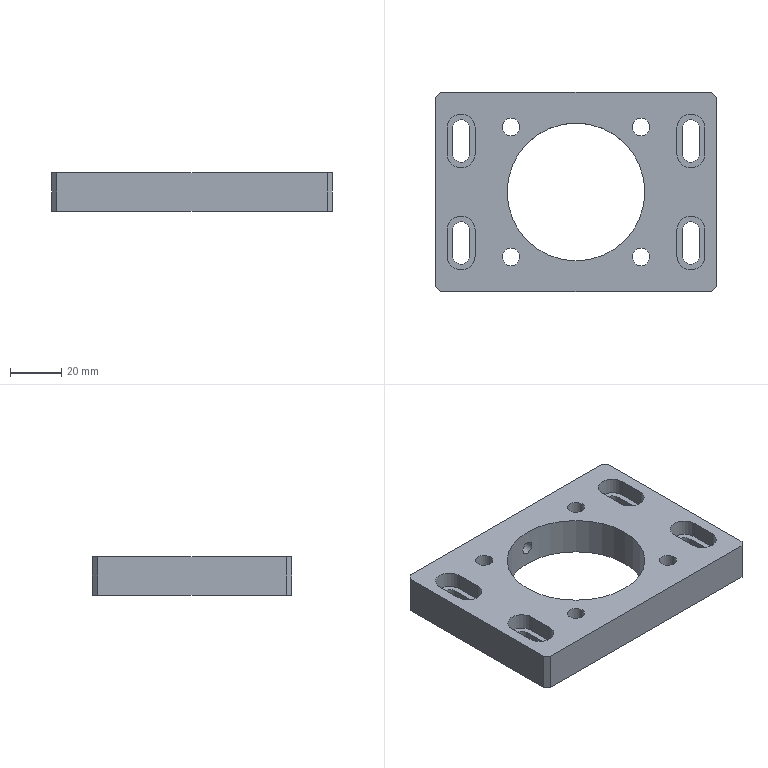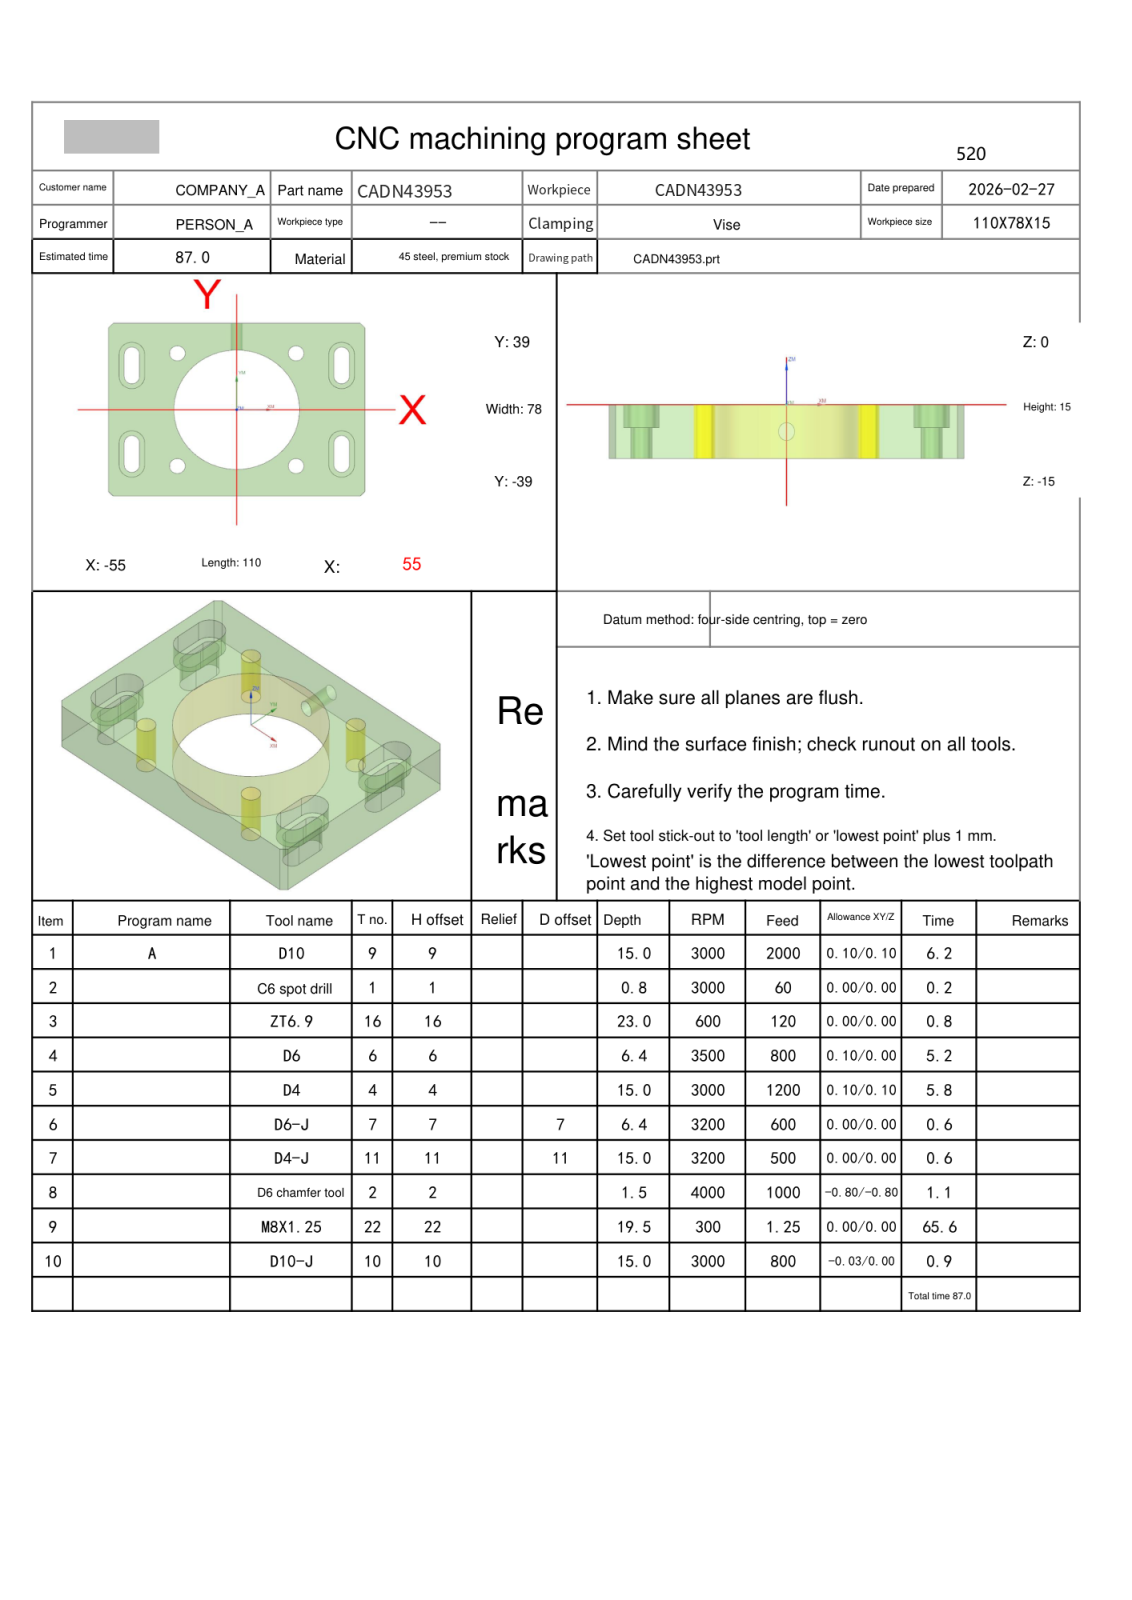NC program | NX | posted by the shop | part box 110 x 78 x 15 mm
Lines 1 to 1524 of 4469:
%
O0001
(Machine time: 151.17 MIN)
(===Total Tool:10===)
(T9=D10     D=10.  R=0.   D-  H09 Z=-15.  )
(T1=C6 spot drill   D=6.   R=0.   D-  H01 Z=-0.8  )
(T16=ZT6.9  D=6.9  DR_a=120 D-  H16 Z=-23.  )
(T6=D6      D=6.   R=0.   D-  H06 Z=-6.4  )
(T4=D4      D=4.   R=0.   D-  H04 Z=-15.  )
(T7=D6-J    D=6.   R=0.   D7  H07 Z=-6.4  )
(T11=D4-J   D=4.   R=0.   D11 H11 Z=-15.  )
(T2=D6 chamfer tool   D=6.   R=0.   D-  H02 Z=-1.5  )
(T22=M8X1.25 D=6.8  DR_a=180 D-  H22 Z=-19.5 )
(T10=D10-J  D=10.  R=0.   D10 H10 Z=-15.  )
G80 G90 G17 G49 G40
G91 G28 Z0
M01
N1 T09 M06
(D10  D=10. R=0. H=09 ce=0.10 di=0.10)
G00 G90 G54 X-50.242 Y-48.97 M03 S3000
G43 H09 Z50.
M08
Z-.5
G01 X-56.606 Y-42.606 F2000.
X-58.606 Y-40.606
X-64.97 Y-34.242
G00 Z-1.
G01 X-58.606 Y-40.606
X-56.606 Y-42.606
X-50.242 Y-48.97
G00 Z-1.5
G01 X-56.606 Y-42.606
X-58.606 Y-40.606
X-64.97 Y-34.242
G00 Z-2.
G01 X-58.606 Y-40.606
X-56.606 Y-42.606
X-50.242 Y-48.97
G00 Z-2.5
G01 X-56.606 Y-42.606
X-58.606 Y-40.606
X-64.97 Y-34.242
G00 Z-3.
G01 X-58.606 Y-40.606
X-56.606 Y-42.606
X-50.242 Y-48.97
G00 Z-3.5
G01 X-56.606 Y-42.606
X-58.606 Y-40.606
X-64.97 Y-34.242
G00 Z-4.
G01 X-58.606 Y-40.606
X-56.606 Y-42.606
X-50.242 Y-48.97
G00 Z-4.5
G01 X-56.606 Y-42.606
X-58.606 Y-40.606
X-64.97 Y-34.242
G00 Z-5.
G01 X-58.606 Y-40.606
X-56.606 Y-42.606
X-50.242 Y-48.97
G00 Z-5.5
G01 X-56.606 Y-42.606
X-58.606 Y-40.606
X-64.97 Y-34.242
G00 Z-6.
G01 X-58.606 Y-40.606
X-56.606 Y-42.606
X-50.242 Y-48.97
G00 Z-6.5
G01 X-56.606 Y-42.606
X-58.606 Y-40.606
X-64.97 Y-34.242
G00 Z-7.
G01 X-58.606 Y-40.606
X-56.606 Y-42.606
X-50.242 Y-48.97
G00 Z-7.5
G01 X-56.606 Y-42.606
X-58.606 Y-40.606
X-64.97 Y-34.242
G00 Z-7.9
G01 X-58.606 Y-40.606
X-56.606 Y-42.606
X-50.242 Y-48.97
G00 Z50.
X-64.97 Y34.242
Z-.5
G01 X-58.606 Y40.606
X-56.606 Y42.606
X-50.242 Y48.97
G00 Z-1.
G01 X-56.606 Y42.606
X-58.606 Y40.606
X-64.97 Y34.242
G00 Z-1.5
G01 X-58.606 Y40.606
X-56.606 Y42.606
X-50.242 Y48.97
G00 Z-2.
G01 X-56.606 Y42.606
X-58.606 Y40.606
X-64.97 Y34.242
G00 Z-2.5
G01 X-58.606 Y40.606
X-56.606 Y42.606
X-50.242 Y48.97
G00 Z-3.
G01 X-56.606 Y42.606
X-58.606 Y40.606
X-64.97 Y34.242
G00 Z-3.5
G01 X-58.606 Y40.606
X-56.606 Y42.606
X-50.242 Y48.97
G00 Z-4.
G01 X-56.606 Y42.606
X-58.606 Y40.606
X-64.97 Y34.242
G00 Z-4.5
G01 X-58.606 Y40.606
X-56.606 Y42.606
X-50.242 Y48.97
G00 Z-5.
G01 X-56.606 Y42.606
X-58.606 Y40.606
X-64.97 Y34.242
G00 Z-5.5
G01 X-58.606 Y40.606
X-56.606 Y42.606
X-50.242 Y48.97
G00 Z-6.
G01 X-56.606 Y42.606
X-58.606 Y40.606
X-64.97 Y34.242
G00 Z-6.5
G01 X-58.606 Y40.606
X-56.606 Y42.606
X-50.242 Y48.97
G00 Z-7.
G01 X-56.606 Y42.606
X-58.606 Y40.606
X-64.97 Y34.242
G00 Z-7.5
G01 X-58.606 Y40.606
X-56.606 Y42.606
X-50.242 Y48.97
G00 Z-7.9
G01 X-56.606 Y42.606
X-58.606 Y40.606
X-64.97 Y34.242
G00 Z50.
X50.242 Y48.97
Z-.5
G01 X56.606 Y42.606
X58.606 Y40.606
X64.97 Y34.242
G00 Z-1.
G01 X58.606 Y40.606
X56.606 Y42.606
X50.242 Y48.97
G00 Z-1.5
G01 X56.606 Y42.606
X58.606 Y40.606
X64.97 Y34.242
G00 Z-2.
G01 X58.606 Y40.606
X56.606 Y42.606
X50.242 Y48.97
G00 Z-2.5
G01 X56.606 Y42.606
X58.606 Y40.606
X64.97 Y34.242
G00 Z-3.
G01 X58.606 Y40.606
X56.606 Y42.606
X50.242 Y48.97
G00 Z-3.5
G01 X56.606 Y42.606
X58.606 Y40.606
X64.97 Y34.242
G00 Z-4.
G01 X58.606 Y40.606
X56.606 Y42.606
X50.242 Y48.97
G00 Z-4.5
G01 X56.606 Y42.606
X58.606 Y40.606
X64.97 Y34.242
G00 Z-5.
G01 X58.606 Y40.606
X56.606 Y42.606
X50.242 Y48.97
G00 Z-5.5
G01 X56.606 Y42.606
X58.606 Y40.606
X64.97 Y34.242
G00 Z-6.
G01 X58.606 Y40.606
X56.606 Y42.606
X50.242 Y48.97
G00 Z-6.5
G01 X56.606 Y42.606
X58.606 Y40.606
X64.97 Y34.242
G00 Z-7.
G01 X58.606 Y40.606
X56.606 Y42.606
X50.242 Y48.97
G00 Z-7.5
G01 X56.606 Y42.606
X58.606 Y40.606
X64.97 Y34.242
G00 Z-7.9
G01 X58.606 Y40.606
X56.606 Y42.606
X50.242 Y48.97
G00 Z50.
X64.97 Y-34.242
Z-.5
G01 X58.606 Y-40.606
X56.606 Y-42.606
X50.242 Y-48.97
G00 Z-1.
G01 X56.606 Y-42.606
X58.606 Y-40.606
X64.97 Y-34.242
G00 Z-1.5
G01 X58.606 Y-40.606
X56.606 Y-42.606
X50.242 Y-48.97
G00 Z-2.
G01 X56.606 Y-42.606
X58.606 Y-40.606
X64.97 Y-34.242
G00 Z-2.5
G01 X58.606 Y-40.606
X56.606 Y-42.606
X50.242 Y-48.97
G00 Z-3.
G01 X56.606 Y-42.606
X58.606 Y-40.606
X64.97 Y-34.242
G00 Z-3.5
G01 X58.606 Y-40.606
X56.606 Y-42.606
X50.242 Y-48.97
G00 Z-4.
G01 X56.606 Y-42.606
X58.606 Y-40.606
X64.97 Y-34.242
G00 Z-4.5
G01 X58.606 Y-40.606
X56.606 Y-42.606
X50.242 Y-48.97
G00 Z-5.
G01 X56.606 Y-42.606
X58.606 Y-40.606
X64.97 Y-34.242
G00 Z-5.5
G01 X58.606 Y-40.606
X56.606 Y-42.606
X50.242 Y-48.97
G00 Z-6.
G01 X56.606 Y-42.606
X58.606 Y-40.606
X64.97 Y-34.242
G00 Z-6.5
G01 X58.606 Y-40.606
X56.606 Y-42.606
X50.242 Y-48.97
G00 Z-7.
G01 X56.606 Y-42.606
X58.606 Y-40.606
X64.97 Y-34.242
G00 Z-7.5
G01 X58.606 Y-40.606
X56.606 Y-42.606
X50.242 Y-48.97
G00 Z-7.9
G01 X56.606 Y-42.606
X58.606 Y-40.606
X64.97 Y-34.242
G00 Z50.
G00 G90 X-1.466 Y12.145 M03 S3000
Z10.1
Z1.5
G02 X-1.466 Y12.145 Z.018 I1.466 J4.255 F2000.
X-2.587 Y20.082 Z-.5 I1.466 J4.255
G01 X0.0 Y21.9
G02 X21.9 Y0.0 I0.0 J-21.9
X0.0 Y-21.9 I-21.9 J0.0
X-21.9 Y0.0 I0.0 J21.9
X0.0 Y21.9 I21.9 J0.0
X4.957 Y21.332 I0.0 J-21.9
X5.73 Y20.36 I-.226 J-.974
G01 X5.747 Y14.394
G03 X6.322 Y13.492 I1. J.003
G02 X14.9 Y0.0 I-6.322 J-13.492
X0.0 Y-14.9 I-14.9 J0.0
X-14.9 Y0.0 I0.0 J14.9
X0.0 Y14.9 I14.9 J0.0
X.225 Y14.898 I0.0 J-14.9
X1.14 Y14.265 I-.015 J-1.
G01 X3.975 Y7.06
G03 X4.354 Y6.592 I.93 J.366
G02 X7.9 Y0.0 I-4.354 J-6.592
X0.0 Y-7.9 I-7.9 J0.0
X-7.9 Y0.0 I0.0 J7.9
X-1.587 Y7.739 I7.9 J0.0
G01 X-1.407 Y7.757
G02 X-.525 Y7.038 I0.0 J-.9
G01 X.873 Y.224
X.88 Y.19
X.9 Y0.0
G02 X0.0 Y-.9 I-.9 J0.0
X-.9 Y0.0 I0.0 J.9
X0.0 Y.9 I.9 J0.0
X.204 Y.877 I0.0 J-.9
X.635 Y.637 I-.204 J-.877
G03 X5.578 Y-1.405 I4.942 J4.957
X10.535 Y.653 I0.0 J7.
G01 Z.7
G00 Z3.
G01 X-1.466 Y12.145 F6000.
G00 Z1.
G02 X-1.466 Y12.145 Z-.482 I1.466 J4.255 F2000.
X-2.587 Y20.082 Z-1. I1.466 J4.255
G01 X0.0 Y21.9
G02 X21.9 Y0.0 I0.0 J-21.9
X0.0 Y-21.9 I-21.9 J0.0
X-21.9 Y0.0 I0.0 J21.9
X0.0 Y21.9 I21.9 J0.0
X4.957 Y21.332 I0.0 J-21.9
X5.73 Y20.36 I-.226 J-.974
G01 X5.747 Y14.394
G03 X6.322 Y13.492 I1. J.003
G02 X14.9 Y0.0 I-6.322 J-13.492
X0.0 Y-14.9 I-14.9 J0.0
X-14.9 Y0.0 I0.0 J14.9
X0.0 Y14.9 I14.9 J0.0
X.225 Y14.898 I0.0 J-14.9
X1.14 Y14.265 I-.015 J-1.
G01 X3.975 Y7.06
G03 X4.354 Y6.592 I.93 J.366
G02 X7.9 Y0.0 I-4.354 J-6.592
X0.0 Y-7.9 I-7.9 J0.0
X-7.9 Y0.0 I0.0 J7.9
X-1.587 Y7.739 I7.9 J0.0
G01 X-1.407 Y7.757
G02 X-.525 Y7.038 I0.0 J-.9
G01 X.873 Y.224
X.88 Y.19
X.9 Y0.0
G02 X0.0 Y-.9 I-.9 J0.0
X-.9 Y0.0 I0.0 J.9
X0.0 Y.9 I.9 J0.0
X.204 Y.877 I0.0 J-.9
X.635 Y.637 I-.204 J-.877
G03 X5.578 Y-1.405 I4.942 J4.957
X10.535 Y.653 I0.0 J7.
G01 Z.2
G00 Z2.5
G01 X-1.466 Y12.145 F6000.
G00 Z.5
G02 X-1.466 Y12.145 Z-.982 I1.466 J4.255 F2000.
X-2.587 Y20.082 Z-1.5 I1.466 J4.255
G01 X0.0 Y21.9
G02 X21.9 Y0.0 I0.0 J-21.9
X0.0 Y-21.9 I-21.9 J0.0
X-21.9 Y0.0 I0.0 J21.9
X0.0 Y21.9 I21.9 J0.0
X4.957 Y21.332 I0.0 J-21.9
X5.73 Y20.36 I-.226 J-.974
G01 X5.747 Y14.394
G03 X6.322 Y13.492 I1. J.003
G02 X14.9 Y0.0 I-6.322 J-13.492
X0.0 Y-14.9 I-14.9 J0.0
X-14.9 Y0.0 I0.0 J14.9
X0.0 Y14.9 I14.9 J0.0
X.225 Y14.898 I0.0 J-14.9
X1.14 Y14.265 I-.015 J-1.
G01 X3.975 Y7.06
G03 X4.354 Y6.592 I.93 J.366
G02 X7.9 Y0.0 I-4.354 J-6.592
X0.0 Y-7.9 I-7.9 J0.0
X-7.9 Y0.0 I0.0 J7.9
X-1.587 Y7.739 I7.9 J0.0
G01 X-1.407 Y7.757
G02 X-.525 Y7.038 I0.0 J-.9
G01 X.872 Y.225
X.88 Y.19
X.9 Y0.0
G02 X0.0 Y-.9 I-.9 J0.0
X-.9 Y0.0 I0.0 J.9
X0.0 Y.9 I.9 J0.0
X.204 Y.877 I0.0 J-.9
G01 X.265 Y.86
G02 X.635 Y.637 I-.265 J-.86
G03 X5.578 Y-1.405 I4.942 J4.957
X10.535 Y.653 I0.0 J7.
G01 Z-.3
G00 Z2.
G01 X-1.466 Y12.145 F6000.
G00 Z0.0
G02 X-1.466 Y12.145 Z-1.482 I1.466 J4.255 F2000.
X-2.587 Y20.082 Z-2. I1.466 J4.255
G01 X0.0 Y21.9
G02 X21.9 Y0.0 I0.0 J-21.9
X0.0 Y-21.9 I-21.9 J0.0
X-21.9 Y0.0 I0.0 J21.9
X0.0 Y21.9 I21.9 J0.0
X4.957 Y21.332 I0.0 J-21.9
X5.73 Y20.36 I-.226 J-.974
G01 X5.747 Y14.394
G03 X6.322 Y13.492 I1. J.003
G02 X14.9 Y0.0 I-6.322 J-13.492
X0.0 Y-14.9 I-14.9 J0.0
X-14.9 Y0.0 I0.0 J14.9
X0.0 Y14.9 I14.9 J0.0
X.225 Y14.898 I0.0 J-14.9
X1.14 Y14.265 I-.015 J-1.
G01 X3.975 Y7.06
G03 X4.354 Y6.592 I.93 J.366
G02 X7.9 Y0.0 I-4.354 J-6.592
X0.0 Y-7.9 I-7.9 J0.0
X-7.9 Y0.0 I0.0 J7.9
X-1.651 Y7.725 I7.9 J0.0
G01 X-1.464 Y7.745
G02 X-.572 Y6.968 I0.0 J-.9
G01 X.095 Y2.097
G03 X.727 Y.531 I3.422 J.469
G02 X.9 Y0.0 I-.727 J-.531
X0.0 Y-.9 I-.9 J0.0
X-.9 Y0.0 I0.0 J.9
X0.0 Y.9 I.9 J0.0
X.204 Y.877 I0.0 J-.9
G01 X.265 Y.86
G02 X.635 Y.637 I-.265 J-.86
G03 X5.578 Y-1.405 I4.942 J4.957
X10.535 Y.653 I0.0 J7.
G01 Z-.8
G00 Z1.5
G01 X-1.466 Y12.145 F6000.
G00 Z-.5
G02 X-1.466 Y12.145 Z-1.982 I1.466 J4.255 F2000.
X-2.587 Y20.082 Z-2.5 I1.466 J4.255
G01 X0.0 Y21.9
G02 X21.9 Y0.0 I0.0 J-21.9
X0.0 Y-21.9 I-21.9 J0.0
X-21.9 Y0.0 I0.0 J21.9
X0.0 Y21.9 I21.9 J0.0
X4.957 Y21.332 I0.0 J-21.9
X5.73 Y20.36 I-.226 J-.974
G01 X5.747 Y14.394
G03 X6.322 Y13.492 I1. J.003
G02 X14.9 Y0.0 I-6.322 J-13.492
X0.0 Y-14.9 I-14.9 J0.0
X-14.9 Y0.0 I0.0 J14.9
X0.0 Y14.9 I14.9 J0.0
X.225 Y14.898 I0.0 J-14.9
X1.14 Y14.265 I-.015 J-1.
G01 X3.975 Y7.06
G03 X4.354 Y6.592 I.93 J.366
G02 X7.9 Y0.0 I-4.354 J-6.592
X0.0 Y-7.9 I-7.9 J0.0
X-7.9 Y0.0 I0.0 J7.9
X-1.628 Y7.731 I7.9 J0.0
G01 X-1.442 Y7.75
G02 X-.554 Y6.994 I0.0 J-.9
G01 X.295 Y1.737
G03 X.766 Y.473 I3.41 J.551
G02 X.9 Y0.0 I-.766 J-.473
X0.0 Y-.9 I-.9 J0.0
X-.9 Y0.0 I0.0 J.9
X0.0 Y.9 I.9 J0.0
X.204 Y.877 I0.0 J-.9
G01 X.265 Y.86
G02 X.635 Y.637 I-.265 J-.86
G03 X5.578 Y-1.405 I4.942 J4.957
X10.535 Y.653 I0.0 J7.
G01 Z-1.3
G00 Z1.
G01 X-1.466 Y12.145 F6000.
G00 Z-1.
G02 X-1.466 Y12.145 Z-2.482 I1.466 J4.255 F2000.
X-2.587 Y20.082 Z-3. I1.466 J4.255
G01 X0.0 Y21.9
G02 X21.9 Y0.0 I0.0 J-21.9
X0.0 Y-21.9 I-21.9 J0.0
X-21.9 Y0.0 I0.0 J21.9
X0.0 Y21.9 I21.9 J0.0
X4.957 Y21.332 I0.0 J-21.9
X5.73 Y20.36 I-.226 J-.974
G01 X5.747 Y14.394
G03 X6.322 Y13.492 I1. J.003
G02 X14.9 Y0.0 I-6.322 J-13.492
X0.0 Y-14.9 I-14.9 J0.0
X-14.9 Y0.0 I0.0 J14.9
X0.0 Y14.9 I14.9 J0.0
X.225 Y14.898 I0.0 J-14.9
X1.14 Y14.265 I-.015 J-1.
G01 X3.975 Y7.06
G03 X4.354 Y6.592 I.93 J.366
G02 X7.9 Y0.0 I-4.354 J-6.592
X0.0 Y-7.9 I-7.9 J0.0
X-7.9 Y0.0 I0.0 J7.9
X-1.651 Y7.725 I7.9 J0.0
G01 X-1.464 Y7.745
G02 X-.572 Y6.968 I0.0 J-.9
G01 X.095 Y2.097
G03 X.727 Y.531 I3.422 J.469
G02 X.9 Y0.0 I-.727 J-.531
X0.0 Y-.9 I-.9 J0.0
X-.9 Y0.0 I0.0 J.9
X0.0 Y.9 I.9 J0.0
X.204 Y.877 I0.0 J-.9
G01 X.265 Y.86
G02 X.635 Y.637 I-.265 J-.86
G03 X5.578 Y-1.405 I4.942 J4.957
X10.535 Y.653 I0.0 J7.
G01 Z-1.8
G00 Z.5
G01 X-1.466 Y12.145 F6000.
G00 Z-1.5
G02 X-1.466 Y12.145 Z-2.982 I1.466 J4.255 F2000.
X-2.587 Y20.082 Z-3.5 I1.466 J4.255
G01 X0.0 Y21.9
G02 X21.9 Y0.0 I0.0 J-21.9
X0.0 Y-21.9 I-21.9 J0.0
X-21.9 Y0.0 I0.0 J21.9
X0.0 Y21.9 I21.9 J0.0
X4.957 Y21.332 I0.0 J-21.9
X5.73 Y20.36 I-.226 J-.974
G01 X5.747 Y14.394
G03 X6.322 Y13.492 I1. J.003
G02 X14.9 Y0.0 I-6.322 J-13.492
X0.0 Y-14.9 I-14.9 J0.0
X-14.9 Y0.0 I0.0 J14.9
X0.0 Y14.9 I14.9 J0.0
X.225 Y14.898 I0.0 J-14.9
X1.14 Y14.265 I-.015 J-1.
G01 X3.975 Y7.06
G03 X4.354 Y6.592 I.93 J.366
G02 X7.9 Y0.0 I-4.354 J-6.592
X0.0 Y-7.9 I-7.9 J0.0
X-7.9 Y0.0 I0.0 J7.9
X-1.651 Y7.725 I7.9 J0.0
G01 X-1.464 Y7.745
G02 X-.572 Y6.968 I0.0 J-.9
G01 X.095 Y2.097
G03 X.727 Y.531 I3.422 J.469
G02 X.9 Y0.0 I-.727 J-.531
X0.0 Y-.9 I-.9 J0.0
X-.9 Y0.0 I0.0 J.9
X0.0 Y.9 I.9 J0.0
X.204 Y.877 I0.0 J-.9
G01 X.265 Y.86
G02 X.635 Y.637 I-.265 J-.86
G03 X5.578 Y-1.405 I4.942 J4.957
X10.535 Y.653 I0.0 J7.
G01 Z-2.3
G00 Z0.0
G01 X-1.466 Y12.145 F6000.
G00 Z-2.
G02 X-1.466 Y12.145 Z-3.482 I1.466 J4.255 F2000.
X-2.587 Y20.082 Z-4. I1.466 J4.255
G01 X0.0 Y21.9
G02 X21.9 Y0.0 I0.0 J-21.9
X0.0 Y-21.9 I-21.9 J0.0
X-21.9 Y0.0 I0.0 J21.9
X0.0 Y21.9 I21.9 J0.0
X4.957 Y21.332 I0.0 J-21.9
X5.73 Y20.36 I-.226 J-.974
G01 X5.747 Y14.394
G03 X6.322 Y13.492 I1. J.003
G02 X14.9 Y0.0 I-6.322 J-13.492
X0.0 Y-14.9 I-14.9 J0.0
X-14.9 Y0.0 I0.0 J14.9
X0.0 Y14.9 I14.9 J0.0
X.225 Y14.898 I0.0 J-14.9
X1.14 Y14.265 I-.015 J-1.
G01 X3.975 Y7.06
G03 X4.354 Y6.592 I.93 J.366
G02 X7.9 Y0.0 I-4.354 J-6.592
X0.0 Y-7.9 I-7.9 J0.0
X-7.9 Y0.0 I0.0 J7.9
X-1.651 Y7.725 I7.9 J0.0
G01 X-1.464 Y7.745
G02 X-.572 Y6.968 I0.0 J-.9
G01 X.095 Y2.097
G03 X.727 Y.531 I3.422 J.469
G02 X.9 Y0.0 I-.727 J-.531
X0.0 Y-.9 I-.9 J0.0
X-.9 Y0.0 I0.0 J.9
X0.0 Y.9 I.9 J0.0
X.204 Y.877 I0.0 J-.9
G01 X.265 Y.86
G02 X.635 Y.637 I-.265 J-.86
G03 X5.578 Y-1.405 I4.942 J4.957
X10.535 Y.653 I0.0 J7.
G01 Z-2.8
G00 Z-.5
G01 X-1.466 Y12.145 F6000.
G00 Z-2.5
G02 X-1.466 Y12.145 Z-3.982 I1.466 J4.255 F2000.
X-2.587 Y20.082 Z-4.5 I1.466 J4.255
G01 X0.0 Y21.9
G02 X21.9 Y0.0 I0.0 J-21.9
X0.0 Y-21.9 I-21.9 J0.0
X-21.9 Y0.0 I0.0 J21.9
X0.0 Y21.9 I21.9 J0.0
X4.957 Y21.332 I0.0 J-21.9
X5.73 Y20.36 I-.226 J-.974
G01 X5.747 Y14.394
G03 X6.322 Y13.492 I1. J.003
G02 X14.9 Y0.0 I-6.322 J-13.492
X0.0 Y-14.9 I-14.9 J0.0
X-14.9 Y0.0 I0.0 J14.9
X0.0 Y14.9 I14.9 J0.0
X.225 Y14.898 I0.0 J-14.9
X1.14 Y14.265 I-.015 J-1.
G01 X3.975 Y7.06
G03 X4.354 Y6.592 I.93 J.366
G02 X7.9 Y0.0 I-4.354 J-6.592
X0.0 Y-7.9 I-7.9 J0.0
X-7.9 Y0.0 I0.0 J7.9
X-1.651 Y7.725 I7.9 J0.0
G01 X-1.464 Y7.745
G02 X-.572 Y6.968 I0.0 J-.9
G01 X.095 Y2.097
G03 X.727 Y.531 I3.422 J.469
G02 X.9 Y0.0 I-.727 J-.531
X0.0 Y-.9 I-.9 J0.0
X-.9 Y0.0 I0.0 J.9
X0.0 Y.9 I.9 J0.0
X.204 Y.877 I0.0 J-.9
G01 X.265 Y.86
G02 X.635 Y.637 I-.265 J-.86
G03 X5.578 Y-1.405 I4.942 J4.957
X10.535 Y.653 I0.0 J7.
G01 Z-3.3
G00 Z-1.
G01 X-1.466 Y12.145 F6000.
G00 Z-3.
G02 X-1.466 Y12.145 Z-4.482 I1.466 J4.255 F2000.
X-2.587 Y20.082 Z-5. I1.466 J4.255
G01 X0.0 Y21.9
G02 X21.9 Y0.0 I0.0 J-21.9
X0.0 Y-21.9 I-21.9 J0.0
X-21.9 Y0.0 I0.0 J21.9
X0.0 Y21.9 I21.9 J0.0
X4.957 Y21.332 I0.0 J-21.9
X5.73 Y20.36 I-.226 J-.974
G01 X5.747 Y14.394
G03 X6.322 Y13.492 I1. J.003
G02 X14.9 Y0.0 I-6.322 J-13.492
X0.0 Y-14.9 I-14.9 J0.0
X-14.9 Y0.0 I0.0 J14.9
X0.0 Y14.9 I14.9 J0.0
X.225 Y14.898 I0.0 J-14.9
X1.14 Y14.265 I-.015 J-1.
G01 X3.975 Y7.06
G03 X4.354 Y6.592 I.93 J.366
G02 X7.9 Y0.0 I-4.354 J-6.592
X0.0 Y-7.9 I-7.9 J0.0
X-7.9 Y0.0 I0.0 J7.9
X-1.651 Y7.725 I7.9 J0.0
G01 X-1.464 Y7.745
G02 X-.572 Y6.968 I0.0 J-.9
G01 X.095 Y2.097
G03 X.727 Y.531 I3.422 J.469
G02 X.9 Y0.0 I-.727 J-.531
X0.0 Y-.9 I-.9 J0.0
X-.9 Y0.0 I0.0 J.9
X0.0 Y.9 I.9 J0.0
X.204 Y.877 I0.0 J-.9
G01 X.265 Y.86
G02 X.635 Y.637 I-.265 J-.86
G03 X5.578 Y-1.405 I4.942 J4.957
X10.535 Y.653 I0.0 J7.
G01 Z-3.8
G00 Z-1.5
G01 X-1.466 Y12.145 F6000.
G00 Z-3.5
G02 X-1.466 Y12.145 Z-4.982 I1.466 J4.255 F2000.
X-2.587 Y20.082 Z-5.5 I1.466 J4.255
G01 X0.0 Y21.9
G02 X21.9 Y0.0 I0.0 J-21.9
X0.0 Y-21.9 I-21.9 J0.0
X-21.9 Y0.0 I0.0 J21.9
X0.0 Y21.9 I21.9 J0.0
X4.957 Y21.332 I0.0 J-21.9
X5.73 Y20.36 I-.226 J-.974
G01 X5.747 Y14.394
G03 X6.322 Y13.492 I1. J.003
G02 X14.9 Y0.0 I-6.322 J-13.492
X0.0 Y-14.9 I-14.9 J0.0
X-14.9 Y0.0 I0.0 J14.9
X0.0 Y14.9 I14.9 J0.0
X.225 Y14.898 I0.0 J-14.9
X1.14 Y14.265 I-.015 J-1.
G01 X3.975 Y7.06
G03 X4.354 Y6.592 I.93 J.366
G02 X7.9 Y0.0 I-4.354 J-6.592
X0.0 Y-7.9 I-7.9 J0.0
X-7.9 Y0.0 I0.0 J7.9
X-1.651 Y7.725 I7.9 J0.0
G01 X-1.464 Y7.745
G02 X-.572 Y6.968 I0.0 J-.9
G01 X.095 Y2.097
G03 X.727 Y.531 I3.422 J.469
G02 X.9 Y0.0 I-.727 J-.531
X0.0 Y-.9 I-.9 J0.0
X-.9 Y0.0 I0.0 J.9
X0.0 Y.9 I.9 J0.0
X.204 Y.877 I0.0 J-.9
G01 X.265 Y.86
G02 X.635 Y.637 I-.265 J-.86
G03 X5.578 Y-1.405 I4.942 J4.957
X10.535 Y.653 I0.0 J7.
G01 Z-4.3
G00 Z-2.
G01 X-1.466 Y12.145 F6000.
G00 Z-4.
G02 X-1.466 Y12.145 Z-5.482 I1.466 J4.255 F2000.
X-2.587 Y20.082 Z-6. I1.466 J4.255
G01 X0.0 Y21.9
G02 X21.9 Y0.0 I0.0 J-21.9
X0.0 Y-21.9 I-21.9 J0.0
X-21.9 Y0.0 I0.0 J21.9
X0.0 Y21.9 I21.9 J0.0
X4.957 Y21.332 I0.0 J-21.9
X5.73 Y20.36 I-.226 J-.974
G01 X5.747 Y14.394
G03 X6.322 Y13.492 I1. J.003
G02 X14.9 Y0.0 I-6.322 J-13.492
X0.0 Y-14.9 I-14.9 J0.0
X-14.9 Y0.0 I0.0 J14.9
X0.0 Y14.9 I14.9 J0.0
X.225 Y14.898 I0.0 J-14.9
X1.14 Y14.265 I-.015 J-1.
G01 X3.975 Y7.06
G03 X4.354 Y6.592 I.93 J.366
G02 X7.9 Y0.0 I-4.354 J-6.592
X0.0 Y-7.9 I-7.9 J0.0
X-7.9 Y0.0 I0.0 J7.9
X-1.651 Y7.725 I7.9 J0.0
G01 X-1.464 Y7.745
G02 X-.572 Y6.968 I0.0 J-.9
G01 X.095 Y2.097
G03 X.727 Y.531 I3.422 J.469
G02 X.9 Y0.0 I-.727 J-.531
X0.0 Y-.9 I-.9 J0.0
X-.9 Y0.0 I0.0 J.9
X0.0 Y.9 I.9 J0.0
X.204 Y.877 I0.0 J-.9
G01 X.265 Y.86
G02 X.635 Y.637 I-.265 J-.86
G03 X5.578 Y-1.405 I4.942 J4.957
X10.535 Y.653 I0.0 J7.
G01 Z-4.8
G00 Z-2.5
G01 X-1.466 Y12.145 F6000.
G00 Z-4.5
G02 X-1.466 Y12.145 Z-5.982 I1.466 J4.255 F2000.
X-2.587 Y20.082 Z-6.5 I1.466 J4.255
G01 X0.0 Y21.9
G02 X21.9 Y0.0 I0.0 J-21.9
X0.0 Y-21.9 I-21.9 J0.0
X-21.9 Y0.0 I0.0 J21.9
X0.0 Y21.9 I21.9 J0.0
X4.957 Y21.332 I0.0 J-21.9
X5.73 Y20.36 I-.226 J-.974
G01 X5.747 Y14.394
G03 X6.322 Y13.492 I1. J.003
G02 X14.9 Y0.0 I-6.322 J-13.492
X0.0 Y-14.9 I-14.9 J0.0
X-14.9 Y0.0 I0.0 J14.9
X0.0 Y14.9 I14.9 J0.0
X.225 Y14.898 I0.0 J-14.9
X1.14 Y14.265 I-.015 J-1.
G01 X3.975 Y7.06
G03 X4.354 Y6.592 I.93 J.366
G02 X7.9 Y0.0 I-4.354 J-6.592
X0.0 Y-7.9 I-7.9 J0.0
X-7.9 Y0.0 I0.0 J7.9
X-1.651 Y7.725 I7.9 J0.0
G01 X-1.464 Y7.745
G02 X-.572 Y6.968 I0.0 J-.9
G01 X.095 Y2.097
G03 X.727 Y.531 I3.422 J.469
G02 X.9 Y0.0 I-.727 J-.531
X0.0 Y-.9 I-.9 J0.0
X-.9 Y0.0 I0.0 J.9
X0.0 Y.9 I.9 J0.0
X.204 Y.877 I0.0 J-.9
G01 X.265 Y.86
G02 X.635 Y.637 I-.265 J-.86
G03 X5.578 Y-1.405 I4.942 J4.957
X10.535 Y.653 I0.0 J7.
G01 Z-5.3
G00 Z-3.
G01 X-1.466 Y12.145 F6000.
G00 Z-5.
G02 X-1.466 Y12.145 Z-6.482 I1.466 J4.255 F2000.
X-2.587 Y20.082 Z-7. I1.466 J4.255
G01 X0.0 Y21.9
G02 X21.9 Y0.0 I0.0 J-21.9
X0.0 Y-21.9 I-21.9 J0.0
X-21.9 Y0.0 I0.0 J21.9
X0.0 Y21.9 I21.9 J0.0
X4.957 Y21.332 I0.0 J-21.9
X5.73 Y20.36 I-.226 J-.974
G01 X5.747 Y14.394
G03 X6.322 Y13.492 I1. J.003
G02 X14.9 Y0.0 I-6.322 J-13.492
X0.0 Y-14.9 I-14.9 J0.0
X-14.9 Y0.0 I0.0 J14.9
X0.0 Y14.9 I14.9 J0.0
X.225 Y14.898 I0.0 J-14.9
X1.14 Y14.265 I-.015 J-1.
G01 X3.975 Y7.06
G03 X4.354 Y6.592 I.93 J.366
G02 X7.9 Y0.0 I-4.354 J-6.592
X0.0 Y-7.9 I-7.9 J0.0
X-7.9 Y0.0 I0.0 J7.9
X-1.651 Y7.725 I7.9 J0.0
G01 X-1.464 Y7.745
G02 X-.572 Y6.968 I0.0 J-.9
G01 X.095 Y2.097
G03 X.727 Y.531 I3.422 J.469
G02 X.9 Y0.0 I-.727 J-.531
X0.0 Y-.9 I-.9 J0.0
X-.9 Y0.0 I0.0 J.9
X0.0 Y.9 I.9 J0.0
X.204 Y.877 I0.0 J-.9
G01 X.265 Y.86
G02 X.635 Y.637 I-.265 J-.86
G03 X5.578 Y-1.405 I4.942 J4.957
X10.535 Y.653 I0.0 J7.
G01 Z-5.8
G00 Z-3.5
G01 X-1.466 Y12.145 F6000.
G00 Z-5.5
G02 X-1.466 Y12.145 Z-6.982 I1.466 J4.255 F2000.
X-2.587 Y20.082 Z-7.5 I1.466 J4.255
G01 X0.0 Y21.9
G02 X21.9 Y0.0 I0.0 J-21.9
X0.0 Y-21.9 I-21.9 J0.0
X-21.9 Y0.0 I0.0 J21.9
X0.0 Y21.9 I21.9 J0.0
X4.957 Y21.332 I0.0 J-21.9
X5.73 Y20.36 I-.226 J-.974
G01 X5.747 Y14.394
G03 X6.322 Y13.492 I1. J.003
G02 X14.9 Y0.0 I-6.322 J-13.492
X0.0 Y-14.9 I-14.9 J0.0
X-14.9 Y0.0 I0.0 J14.9
X0.0 Y14.9 I14.9 J0.0
X.225 Y14.898 I0.0 J-14.9
X1.14 Y14.265 I-.015 J-1.
G01 X3.975 Y7.06
G03 X4.354 Y6.592 I.93 J.366
G02 X7.9 Y0.0 I-4.354 J-6.592
X0.0 Y-7.9 I-7.9 J0.0
X-7.9 Y0.0 I0.0 J7.9
X-1.651 Y7.725 I7.9 J0.0
G01 X-1.464 Y7.745
G02 X-.572 Y6.968 I0.0 J-.9
G01 X.095 Y2.097
G03 X.727 Y.531 I3.422 J.469
G02 X.9 Y0.0 I-.727 J-.531
X0.0 Y-.9 I-.9 J0.0
X-.9 Y0.0 I0.0 J.9
X0.0 Y.9 I.9 J0.0
X.204 Y.877 I0.0 J-.9
G01 X.265 Y.86
G02 X.635 Y.637 I-.265 J-.86
G03 X5.578 Y-1.405 I4.942 J4.957
X10.535 Y.653 I0.0 J7.
G01 Z-6.3
G00 Z-4.
G01 X-1.466 Y12.145 F6000.
G00 Z-6.
G02 X-1.466 Y12.145 Z-7.482 I1.466 J4.255 F2000.
X-2.587 Y20.082 Z-8. I1.466 J4.255
G01 X0.0 Y21.9
G02 X21.9 Y0.0 I0.0 J-21.9
X0.0 Y-21.9 I-21.9 J0.0
X-21.9 Y0.0 I0.0 J21.9
X0.0 Y21.9 I21.9 J0.0
X4.957 Y21.332 I0.0 J-21.9
X5.73 Y20.36 I-.226 J-.974
G01 X5.747 Y14.394
G03 X6.322 Y13.492 I1. J.003
G02 X14.9 Y0.0 I-6.322 J-13.492
X0.0 Y-14.9 I-14.9 J0.0
X-14.9 Y0.0 I0.0 J14.9
X0.0 Y14.9 I14.9 J0.0
X.225 Y14.898 I0.0 J-14.9
X1.14 Y14.265 I-.015 J-1.
G01 X3.975 Y7.06
G03 X4.354 Y6.592 I.93 J.366
G02 X7.9 Y0.0 I-4.354 J-6.592
X0.0 Y-7.9 I-7.9 J0.0
X-7.9 Y0.0 I0.0 J7.9
X-1.651 Y7.725 I7.9 J0.0
G01 X-1.464 Y7.745
G02 X-.572 Y6.968 I0.0 J-.9
G01 X.095 Y2.097
G03 X.727 Y.531 I3.422 J.469
G02 X.9 Y0.0 I-.727 J-.531
X0.0 Y-.9 I-.9 J0.0
X-.9 Y0.0 I0.0 J.9
X0.0 Y.9 I.9 J0.0
X.204 Y.877 I0.0 J-.9
G01 X.265 Y.86
G02 X.635 Y.637 I-.265 J-.86
G03 X5.578 Y-1.405 I4.942 J4.957
X10.535 Y.653 I0.0 J7.
G01 Z-6.8
G00 Z-4.5
G01 X-1.466 Y12.145 F6000.
G00 Z-6.5
G02 X-1.466 Y12.145 Z-7.982 I1.466 J4.255 F2000.
X-2.587 Y20.082 Z-8.5 I1.466 J4.255
G01 X0.0 Y21.9
G02 X21.9 Y0.0 I0.0 J-21.9
X0.0 Y-21.9 I-21.9 J0.0
X-21.9 Y0.0 I0.0 J21.9
X0.0 Y21.9 I21.9 J0.0
X4.957 Y21.332 I0.0 J-21.9
X5.73 Y20.36 I-.226 J-.974
G01 X5.747 Y14.394
G03 X6.322 Y13.492 I1. J.003
G02 X14.9 Y0.0 I-6.322 J-13.492
X0.0 Y-14.9 I-14.9 J0.0
X-14.9 Y0.0 I0.0 J14.9
X0.0 Y14.9 I14.9 J0.0
X.225 Y14.898 I0.0 J-14.9
X1.14 Y14.265 I-.015 J-1.
G01 X3.975 Y7.06
G03 X4.354 Y6.592 I.93 J.366
G02 X7.9 Y0.0 I-4.354 J-6.592
X0.0 Y-7.9 I-7.9 J0.0
X-7.9 Y0.0 I0.0 J7.9
X-1.651 Y7.725 I7.9 J0.0
G01 X-1.464 Y7.745
G02 X-.572 Y6.968 I0.0 J-.9
G01 X.095 Y2.097
G03 X.727 Y.531 I3.422 J.469
G02 X.9 Y0.0 I-.727 J-.531
X0.0 Y-.9 I-.9 J0.0
X-.9 Y0.0 I0.0 J.9
X0.0 Y.9 I.9 J0.0
X.204 Y.877 I0.0 J-.9
G01 X.265 Y.86
G02 X.635 Y.637 I-.265 J-.86
G03 X5.578 Y-1.405 I4.942 J4.957
X10.535 Y.653 I0.0 J7.
G01 Z-7.3
G00 Z-5.
G01 X-1.466 Y12.145 F6000.
G00 Z-7.
G02 X-1.466 Y12.145 Z-8.482 I1.466 J4.255 F2000.
X-2.587 Y20.082 Z-9. I1.466 J4.255
G01 X0.0 Y21.9
G02 X21.9 Y0.0 I0.0 J-21.9
X0.0 Y-21.9 I-21.9 J0.0
X-21.9 Y0.0 I0.0 J21.9
X0.0 Y21.9 I21.9 J0.0
X4.957 Y21.332 I0.0 J-21.9
X5.73 Y20.36 I-.226 J-.974
G01 X5.747 Y14.394
G03 X6.322 Y13.492 I1. J.003
G02 X14.9 Y0.0 I-6.322 J-13.492
X0.0 Y-14.9 I-14.9 J0.0
X-14.9 Y0.0 I0.0 J14.9
X0.0 Y14.9 I14.9 J0.0
X.225 Y14.898 I0.0 J-14.9
X1.14 Y14.265 I-.015 J-1.
G01 X3.975 Y7.06
G03 X4.354 Y6.592 I.93 J.366
G02 X7.9 Y0.0 I-4.354 J-6.592
X0.0 Y-7.9 I-7.9 J0.0
X-7.9 Y0.0 I0.0 J7.9
X-1.651 Y7.725 I7.9 J0.0
G01 X-1.464 Y7.745
G02 X-.572 Y6.968 I0.0 J-.9
G01 X.095 Y2.097
G03 X.727 Y.531 I3.422 J.469
G02 X.9 Y0.0 I-.727 J-.531
X0.0 Y-.9 I-.9 J0.0
X-.9 Y0.0 I0.0 J.9
X0.0 Y.9 I.9 J0.0
X.204 Y.877 I0.0 J-.9
G01 X.265 Y.86
G02 X.635 Y.637 I-.265 J-.86
G03 X5.578 Y-1.405 I4.942 J4.957
X10.535 Y.653 I0.0 J7.
G01 Z-7.8
G00 Z-5.5
G01 X-1.466 Y12.145 F6000.
G00 Z-7.5
G02 X-1.466 Y12.145 Z-8.982 I1.466 J4.255 F2000.
X-2.587 Y20.082 Z-9.5 I1.466 J4.255
G01 X0.0 Y21.9
G02 X21.9 Y0.0 I0.0 J-21.9
X0.0 Y-21.9 I-21.9 J0.0
X-21.9 Y0.0 I0.0 J21.9
X0.0 Y21.9 I21.9 J0.0
X4.957 Y21.332 I0.0 J-21.9
X5.73 Y20.36 I-.226 J-.974
G01 X5.747 Y14.394
G03 X6.322 Y13.492 I1. J.003
G02 X14.9 Y0.0 I-6.322 J-13.492
X0.0 Y-14.9 I-14.9 J0.0
X-14.9 Y0.0 I0.0 J14.9
X0.0 Y14.9 I14.9 J0.0
X.225 Y14.898 I0.0 J-14.9
X1.14 Y14.265 I-.015 J-1.
G01 X3.975 Y7.06
G03 X4.354 Y6.592 I.93 J.366
G02 X7.9 Y0.0 I-4.354 J-6.592
X0.0 Y-7.9 I-7.9 J0.0
X-7.9 Y0.0 I0.0 J7.9
X-1.651 Y7.725 I7.9 J0.0
G01 X-1.464 Y7.745
G02 X-.572 Y6.968 I0.0 J-.9
G01 X.095 Y2.097
G03 X.727 Y.531 I3.422 J.469
G02 X.9 Y0.0 I-.727 J-.531
X0.0 Y-.9 I-.9 J0.0
X-.9 Y0.0 I0.0 J.9
X0.0 Y.9 I.9 J0.0
X.204 Y.877 I0.0 J-.9
G01 X.265 Y.86
G02 X.635 Y.637 I-.265 J-.86
G03 X5.578 Y-1.405 I4.942 J4.957
X10.535 Y.653 I0.0 J7.
G01 Z-8.3
G00 Z-6.
G01 X-1.466 Y12.145 F6000.
G00 Z-8.
G02 X-1.466 Y12.145 Z-9.482 I1.466 J4.255 F2000.
X-2.587 Y20.082 Z-10. I1.466 J4.255
G01 X0.0 Y21.9
G02 X21.9 Y0.0 I0.0 J-21.9
X0.0 Y-21.9 I-21.9 J0.0
X-21.9 Y0.0 I0.0 J21.9
X0.0 Y21.9 I21.9 J0.0
X4.957 Y21.332 I0.0 J-21.9
X5.73 Y20.36 I-.226 J-.974
G01 X5.747 Y14.394
G03 X6.322 Y13.492 I1. J.003
G02 X14.9 Y0.0 I-6.322 J-13.492
X0.0 Y-14.9 I-14.9 J0.0
X-14.9 Y0.0 I0.0 J14.9
X0.0 Y14.9 I14.9 J0.0
X.225 Y14.898 I0.0 J-14.9
X1.14 Y14.265 I-.015 J-1.
G01 X3.975 Y7.06
G03 X4.354 Y6.592 I.93 J.366
G02 X7.9 Y0.0 I-4.354 J-6.592
X0.0 Y-7.9 I-7.9 J0.0
X-7.9 Y0.0 I0.0 J7.9
X-1.651 Y7.725 I7.9 J0.0
G01 X-1.464 Y7.745
G02 X-.572 Y6.968 I0.0 J-.9
G01 X.095 Y2.097
G03 X.727 Y.531 I3.422 J.469
G02 X.9 Y0.0 I-.727 J-.531
X0.0 Y-.9 I-.9 J0.0
X-.9 Y0.0 I0.0 J.9
X0.0 Y.9 I.9 J0.0
X.204 Y.877 I0.0 J-.9
G01 X.265 Y.86
G02 X.635 Y.637 I-.265 J-.86
G03 X5.578 Y-1.405 I4.942 J4.957
X10.535 Y.653 I0.0 J7.
G01 Z-8.8
G00 Z-6.5
G01 X-1.466 Y12.145 F6000.
G00 Z-8.5
G02 X-1.466 Y12.145 Z-9.982 I1.466 J4.255 F2000.
X-2.587 Y20.082 Z-10.5 I1.466 J4.255
G01 X0.0 Y21.9
G02 X21.9 Y0.0 I0.0 J-21.9
X0.0 Y-21.9 I-21.9 J0.0
X-21.9 Y0.0 I0.0 J21.9
X0.0 Y21.9 I21.9 J0.0
X4.957 Y21.332 I0.0 J-21.9
X5.73 Y20.36 I-.226 J-.974
G01 X5.747 Y14.394
G03 X6.322 Y13.492 I1. J.003
G02 X14.9 Y0.0 I-6.322 J-13.492
X0.0 Y-14.9 I-14.9 J0.0
X-14.9 Y0.0 I0.0 J14.9
X0.0 Y14.9 I14.9 J0.0
X.225 Y14.898 I0.0 J-14.9
X1.14 Y14.265 I-.015 J-1.
G01 X3.975 Y7.06
G03 X4.354 Y6.592 I.93 J.366
G02 X7.9 Y0.0 I-4.354 J-6.592
X0.0 Y-7.9 I-7.9 J0.0
X-7.9 Y0.0 I0.0 J7.9
X-1.651 Y7.725 I7.9 J0.0
G01 X-1.464 Y7.745
G02 X-.572 Y6.968 I0.0 J-.9
G01 X.095 Y2.097
G03 X.727 Y.531 I3.422 J.469
G02 X.9 Y0.0 I-.727 J-.531
X0.0 Y-.9 I-.9 J0.0
X-.9 Y0.0 I0.0 J.9
X0.0 Y.9 I.9 J0.0
X.204 Y.877 I0.0 J-.9
G01 X.265 Y.86
G02 X.635 Y.637 I-.265 J-.86
G03 X5.578 Y-1.405 I4.942 J4.957
X10.535 Y.653 I0.0 J7.
G01 Z-9.3
G00 Z-7.
G01 X-1.466 Y12.145 F6000.
G00 Z-9.
G02 X-1.466 Y12.145 Z-10.482 I1.466 J4.255 F2000.
X-2.587 Y20.082 Z-11. I1.466 J4.255
G01 X0.0 Y21.9
G02 X21.9 Y0.0 I0.0 J-21.9
X0.0 Y-21.9 I-21.9 J0.0
X-21.9 Y0.0 I0.0 J21.9
X0.0 Y21.9 I21.9 J0.0
X4.957 Y21.332 I0.0 J-21.9
X5.73 Y20.36 I-.226 J-.974
G01 X5.747 Y14.394
G03 X6.322 Y13.492 I1. J.003
G02 X14.9 Y0.0 I-6.322 J-13.492
X0.0 Y-14.9 I-14.9 J0.0
X-14.9 Y0.0 I0.0 J14.9
X0.0 Y14.9 I14.9 J0.0
X.225 Y14.898 I0.0 J-14.9
X1.14 Y14.265 I-.015 J-1.
G01 X3.975 Y7.06
G03 X4.354 Y6.592 I.93 J.366
G02 X7.9 Y0.0 I-4.354 J-6.592
X0.0 Y-7.9 I-7.9 J0.0
X-7.9 Y0.0 I0.0 J7.9
X-1.651 Y7.725 I7.9 J0.0
G01 X-1.464 Y7.745
G02 X-.572 Y6.968 I0.0 J-.9
G01 X.095 Y2.097
G03 X.727 Y.531 I3.422 J.469
G02 X.9 Y0.0 I-.727 J-.531
X0.0 Y-.9 I-.9 J0.0
X-.9 Y0.0 I0.0 J.9
X0.0 Y.9 I.9 J0.0
X.204 Y.877 I0.0 J-.9
G01 X.265 Y.86
G02 X.635 Y.637 I-.265 J-.86
G03 X5.578 Y-1.405 I4.942 J4.957
X10.535 Y.653 I0.0 J7.
G01 Z-9.8
G00 Z-7.5
G01 X-1.466 Y12.145 F6000.
G00 Z-9.5
G02 X-1.466 Y12.145 Z-10.982 I1.466 J4.255 F2000.
X-2.587 Y20.082 Z-11.5 I1.466 J4.255
G01 X0.0 Y21.9
G02 X21.9 Y0.0 I0.0 J-21.9
X0.0 Y-21.9 I-21.9 J0.0
X-21.9 Y0.0 I0.0 J21.9
X0.0 Y21.9 I21.9 J0.0
X4.957 Y21.332 I0.0 J-21.9
X5.73 Y20.36 I-.226 J-.974
G01 X5.747 Y14.394
G03 X6.322 Y13.492 I1. J.003
G02 X14.9 Y0.0 I-6.322 J-13.492
X0.0 Y-14.9 I-14.9 J0.0
X-14.9 Y0.0 I0.0 J14.9
X0.0 Y14.9 I14.9 J0.0
X.225 Y14.898 I0.0 J-14.9
X1.14 Y14.265 I-.015 J-1.
G01 X3.975 Y7.06
G03 X4.354 Y6.592 I.93 J.366
G02 X7.9 Y0.0 I-4.354 J-6.592
X0.0 Y-7.9 I-7.9 J0.0
X-7.9 Y0.0 I0.0 J7.9
X-1.651 Y7.725 I7.9 J0.0
G01 X-1.464 Y7.745
G02 X-.572 Y6.968 I0.0 J-.9
G01 X.095 Y2.097
G03 X.727 Y.531 I3.422 J.469
G02 X.9 Y0.0 I-.727 J-.531
X0.0 Y-.9 I-.9 J0.0
X-.9 Y0.0 I0.0 J.9
X0.0 Y.9 I.9 J0.0
X.204 Y.877 I0.0 J-.9
G01 X.265 Y.86
G02 X.635 Y.637 I-.265 J-.86
G03 X5.578 Y-1.405 I4.942 J4.957
X10.535 Y.653 I0.0 J7.
G01 Z-10.3
G00 Z-8.
G01 X-1.466 Y12.145 F6000.
G00 Z-10.
G02 X-1.466 Y12.145 Z-11.482 I1.466 J4.255 F2000.
X-2.587 Y20.082 Z-12. I1.466 J4.255
G01 X0.0 Y21.9
G02 X21.9 Y0.0 I0.0 J-21.9
X0.0 Y-21.9 I-21.9 J0.0
X-21.9 Y0.0 I0.0 J21.9
X0.0 Y21.9 I21.9 J0.0
X4.957 Y21.332 I0.0 J-21.9
X5.73 Y20.36 I-.226 J-.974
G01 X5.747 Y14.394
G03 X6.322 Y13.492 I1. J.003
G02 X14.9 Y0.0 I-6.322 J-13.492
X0.0 Y-14.9 I-14.9 J0.0
X-14.9 Y0.0 I0.0 J14.9
X0.0 Y14.9 I14.9 J0.0
X.225 Y14.898 I0.0 J-14.9
X1.14 Y14.265 I-.015 J-1.
G01 X3.975 Y7.06
G03 X4.354 Y6.592 I.93 J.366
G02 X7.9 Y0.0 I-4.354 J-6.592
X0.0 Y-7.9 I-7.9 J0.0
X-7.9 Y0.0 I0.0 J7.9
X-1.651 Y7.725 I7.9 J0.0
G01 X-1.464 Y7.745
G02 X-.572 Y6.968 I0.0 J-.9
G01 X.095 Y2.097
G03 X.727 Y.531 I3.422 J.469
G02 X.9 Y0.0 I-.727 J-.531
X0.0 Y-.9 I-.9 J0.0
X-.9 Y0.0 I0.0 J.9
X0.0 Y.9 I.9 J0.0
X.204 Y.877 I0.0 J-.9
G01 X.265 Y.86
G02 X.635 Y.637 I-.265 J-.86
G03 X5.578 Y-1.405 I4.942 J4.957
X10.535 Y.653 I0.0 J7.
G01 Z-10.8
G00 Z-8.5
G01 X-1.466 Y12.145 F6000.
G00 Z-10.5
G02 X-1.466 Y12.145 Z-11.982 I1.466 J4.255 F2000.
X-2.587 Y20.082 Z-12.5 I1.466 J4.255
G01 X0.0 Y21.9
G02 X21.9 Y0.0 I0.0 J-21.9
X0.0 Y-21.9 I-21.9 J0.0
X-21.9 Y0.0 I0.0 J21.9
X0.0 Y21.9 I21.9 J0.0
X4.957 Y21.332 I0.0 J-21.9
X5.73 Y20.36 I-.226 J-.974
G01 X5.747 Y14.394
G03 X6.322 Y13.492 I1. J.003
G02 X14.9 Y0.0 I-6.322 J-13.492
X0.0 Y-14.9 I-14.9 J0.0
X-14.9 Y0.0 I0.0 J14.9
X0.0 Y14.9 I14.9 J0.0
X.225 Y14.898 I0.0 J-14.9
X1.14 Y14.265 I-.015 J-1.
G01 X3.975 Y7.06
G03 X4.354 Y6.592 I.93 J.366
G02 X7.9 Y0.0 I-4.354 J-6.592
X0.0 Y-7.9 I-7.9 J0.0
X-7.9 Y0.0 I0.0 J7.9
X-1.651 Y7.725 I7.9 J0.0
G01 X-1.464 Y7.745
G02 X-.572 Y6.968 I0.0 J-.9
G01 X.095 Y2.097
G03 X.727 Y.531 I3.422 J.469
G02 X.9 Y0.0 I-.727 J-.531
X0.0 Y-.9 I-.9 J0.0
X-.9 Y0.0 I0.0 J.9
X0.0 Y.9 I.9 J0.0
X.204 Y.877 I0.0 J-.9
G01 X.265 Y.86
G02 X.635 Y.637 I-.265 J-.86
G03 X5.578 Y-1.405 I4.942 J4.957
X10.535 Y.653 I0.0 J7.
G01 Z-11.3
G00 Z-9.
G01 X-1.466 Y12.145 F6000.
G00 Z-11.
G02 X-1.466 Y12.145 Z-12.482 I1.466 J4.255 F2000.
X-2.587 Y20.082 Z-13. I1.466 J4.255
G01 X0.0 Y21.9
G02 X21.9 Y0.0 I0.0 J-21.9
X0.0 Y-21.9 I-21.9 J0.0
X-21.9 Y0.0 I0.0 J21.9
X0.0 Y21.9 I21.9 J0.0
X4.957 Y21.332 I0.0 J-21.9
X5.73 Y20.36 I-.226 J-.974
G01 X5.747 Y14.394
G03 X6.322 Y13.492 I1. J.003
G02 X14.9 Y0.0 I-6.322 J-13.492
X0.0 Y-14.9 I-14.9 J0.0
X-14.9 Y0.0 I0.0 J14.9
X0.0 Y14.9 I14.9 J0.0
X.225 Y14.898 I0.0 J-14.9
X1.14 Y14.265 I-.015 J-1.
G01 X3.975 Y7.06
G03 X4.354 Y6.592 I.93 J.366
G02 X7.9 Y0.0 I-4.354 J-6.592
X0.0 Y-7.9 I-7.9 J0.0
X-7.9 Y0.0 I0.0 J7.9
X-1.651 Y7.725 I7.9 J0.0
G01 X-1.464 Y7.745
G02 X-.572 Y6.968 I0.0 J-.9
G01 X.095 Y2.097
G03 X.727 Y.531 I3.422 J.469
G02 X.9 Y0.0 I-.727 J-.531
X0.0 Y-.9 I-.9 J0.0
X-.9 Y0.0 I0.0 J.9
X0.0 Y.9 I.9 J0.0
X.204 Y.877 I0.0 J-.9
G01 X.265 Y.86
G02 X.635 Y.637 I-.265 J-.86
G03 X5.578 Y-1.405 I4.942 J4.957
X10.535 Y.653 I0.0 J7.
G01 Z-11.8
G00 Z-9.5
G01 X-1.466 Y12.145 F6000.
G00 Z-11.5
G02 X-1.466 Y12.145 Z-12.982 I1.466 J4.255 F2000.
X-2.587 Y20.082 Z-13.5 I1.466 J4.255
G01 X0.0 Y21.9
G02 X21.9 Y0.0 I0.0 J-21.9
X0.0 Y-21.9 I-21.9 J0.0
X-21.9 Y0.0 I0.0 J21.9
X0.0 Y21.9 I21.9 J0.0
X4.957 Y21.332 I0.0 J-21.9
X5.73 Y20.36 I-.226 J-.974
G01 X5.747 Y14.394
G03 X6.322 Y13.492 I1. J.003
G02 X14.9 Y0.0 I-6.322 J-13.492
X0.0 Y-14.9 I-14.9 J0.0
X-14.9 Y0.0 I0.0 J14.9
X0.0 Y14.9 I14.9 J0.0
X.225 Y14.898 I0.0 J-14.9
X1.14 Y14.265 I-.015 J-1.
G01 X3.975 Y7.06
G03 X4.354 Y6.592 I.93 J.366
G02 X7.9 Y0.0 I-4.354 J-6.592
X0.0 Y-7.9 I-7.9 J0.0
X-7.9 Y0.0 I0.0 J7.9
X-1.651 Y7.725 I7.9 J0.0
G01 X-1.464 Y7.745
G02 X-.572 Y6.968 I0.0 J-.9
G01 X.095 Y2.097
G03 X.727 Y.531 I3.422 J.469
G02 X.9 Y0.0 I-.727 J-.531
X0.0 Y-.9 I-.9 J0.0
X-.9 Y0.0 I0.0 J.9
X0.0 Y.9 I.9 J0.0
X.204 Y.877 I0.0 J-.9
G01 X.265 Y.86
G02 X.635 Y.637 I-.265 J-.86
G03 X5.578 Y-1.405 I4.942 J4.957
X10.535 Y.653 I0.0 J7.
G01 Z-12.3
G00 Z-10.
G01 X-1.466 Y12.145 F6000.
G00 Z-12.
G02 X-1.466 Y12.145 Z-13.482 I1.466 J4.255 F2000.
X-2.587 Y20.082 Z-14. I1.466 J4.255
G01 X0.0 Y21.9
G02 X21.9 Y0.0 I0.0 J-21.9
X0.0 Y-21.9 I-21.9 J0.0
X-21.9 Y0.0 I0.0 J21.9
X0.0 Y21.9 I21.9 J0.0
X4.957 Y21.332 I0.0 J-21.9
X5.73 Y20.36 I-.226 J-.974
G01 X5.747 Y14.394
G03 X6.322 Y13.492 I1. J.003
G02 X14.9 Y0.0 I-6.322 J-13.492
X0.0 Y-14.9 I-14.9 J0.0
X-14.9 Y0.0 I0.0 J14.9
X0.0 Y14.9 I14.9 J0.0
X.225 Y14.898 I0.0 J-14.9
X1.14 Y14.265 I-.015 J-1.
G01 X3.975 Y7.06
G03 X4.354 Y6.592 I.93 J.366
G02 X7.9 Y0.0 I-4.354 J-6.592
X0.0 Y-7.9 I-7.9 J0.0
X-7.9 Y0.0 I0.0 J7.9
X-1.651 Y7.725 I7.9 J0.0
G01 X-1.464 Y7.745
G02 X-.572 Y6.968 I0.0 J-.9
G01 X.095 Y2.097
G03 X.727 Y.531 I3.422 J.469
G02 X.9 Y0.0 I-.727 J-.531
X0.0 Y-.9 I-.9 J0.0
X-.9 Y0.0 I0.0 J.9
X0.0 Y.9 I.9 J0.0
X.204 Y.877 I0.0 J-.9
G01 X.265 Y.86
G02 X.635 Y.637 I-.265 J-.86
G03 X5.578 Y-1.405 I4.942 J4.957
X10.535 Y.653 I0.0 J7.
G01 Z-12.8
G00 Z-10.5
G01 X-1.466 Y12.145 F6000.
G00 Z-12.5
G02 X-1.466 Y12.145 Z-13.982 I1.466 J4.255 F2000.
X-2.587 Y20.082 Z-14.5 I1.466 J4.255
G01 X0.0 Y21.9
G02 X21.9 Y0.0 I0.0 J-21.9
X0.0 Y-21.9 I-21.9 J0.0
X-21.9 Y0.0 I0.0 J21.9
X0.0 Y21.9 I21.9 J0.0
X4.957 Y21.332 I0.0 J-21.9
X5.73 Y20.36 I-.226 J-.974
G01 X5.747 Y14.394
G03 X6.322 Y13.492 I1. J.003
G02 X14.9 Y0.0 I-6.322 J-13.492
X0.0 Y-14.9 I-14.9 J0.0
X-14.9 Y0.0 I0.0 J14.9
X0.0 Y14.9 I14.9 J0.0
X.225 Y14.898 I0.0 J-14.9
X1.14 Y14.265 I-.015 J-1.
G01 X3.975 Y7.06
G03 X4.354 Y6.592 I.93 J.366
G02 X7.9 Y0.0 I-4.354 J-6.592
X0.0 Y-7.9 I-7.9 J0.0
X-7.9 Y0.0 I0.0 J7.9
X-1.651 Y7.725 I7.9 J0.0
G01 X-1.464 Y7.745
G02 X-.572 Y6.968 I0.0 J-.9
G01 X.095 Y2.097
G03 X.727 Y.531 I3.422 J.469
G02 X.9 Y0.0 I-.727 J-.531
X0.0 Y-.9 I-.9 J0.0
X-.9 Y0.0 I0.0 J.9
X0.0 Y.9 I.9 J0.0
X.204 Y.877 I0.0 J-.9
G01 X.265 Y.86
G02 X.635 Y.637 I-.265 J-.86
G03 X5.578 Y-1.405 I4.942 J4.957
X10.535 Y.653 I0.0 J7.
G01 Z-13.3
G00 Z-11.
G01 X-1.466 Y12.145 F6000.
G00 Z-13.
G02 X-1.466 Y12.145 Z-14.482 I1.466 J4.255 F2000.
X-2.587 Y20.082 Z-15. I1.466 J4.255
G01 X0.0 Y21.9
G02 X21.9 Y0.0 I0.0 J-21.9
X0.0 Y-21.9 I-21.9 J0.0
X-21.9 Y0.0 I0.0 J21.9
X0.0 Y21.9 I21.9 J0.0
X4.957 Y21.332 I0.0 J-21.9
X5.73 Y20.36 I-.226 J-.974
G01 X5.747 Y14.394
G03 X6.322 Y13.492 I1. J.003
G02 X14.9 Y0.0 I-6.322 J-13.492
X0.0 Y-14.9 I-14.9 J0.0
X-14.9 Y0.0 I0.0 J14.9
X0.0 Y14.9 I14.9 J0.0
X.225 Y14.898 I0.0 J-14.9
X1.14 Y14.265 I-.015 J-1.
G01 X3.975 Y7.06
G03 X4.354 Y6.592 I.93 J.366
G02 X7.9 Y0.0 I-4.354 J-6.592
X0.0 Y-7.9 I-7.9 J0.0
X-7.9 Y0.0 I0.0 J7.9
X-1.59 Y7.738 I7.9 J0.0
G01 X-1.409 Y7.757
G02 X-.527 Y7.035 I0.0 J-.9
G01 X.762 Y.64
G03 X.857 Y.274 I3.386 J.683
G02 X.9 Y0.0 I-.857 J-.274
X0.0 Y-.9 I-.9 J0.0
X-.9 Y0.0 I0.0 J.9
X0.0 Y.9 I.9 J0.0
X.204 Y.877 I0.0 J-.9
G01 X.265 Y.86
G02 X.635 Y.637 I-.265 J-.86
G03 X5.578 Y-1.405 I4.942 J4.957
X10.535 Y.653 I0.0 J7.
G01 Z-13.8
G00 Z10.1
G91 G28 Z0.0
M05
M09
G91 G28 Z0.0
M01
N2 T01 M06
(C6 spot drill  D=6. R=0. H=01 ce=0.00 di=0.10)
G00 G90 G54 X25.456 Y25.456 M03 S3000
G43 H01 Z50.
M08
G98 G81 X25.456 Y25.456 Z-.8 R1. F60.
Y-25.456
X0.0 Y0.0
X-25.456 Y-25.456
Y25.456
G80
G00 Z50.
G91 G28 Z0.0
M05
M09
G91 G28 Z0.0
M01
N3 T16 M06
(ZT6.9 D=6.9 DR_a=120 H=16)
G00 G90 G54 X25.456 Y25.456 M03 S600
G43 H16 Z50.
M08
G98 G83 X25.456 Y25.456 Z-23. R1. F120. Q2.
Y-25.456
X-25.456
Y25.456
G80
G00 Z50.
G91 G28 Z0.0
M05
M09
G91 G28 Z0.0
M01